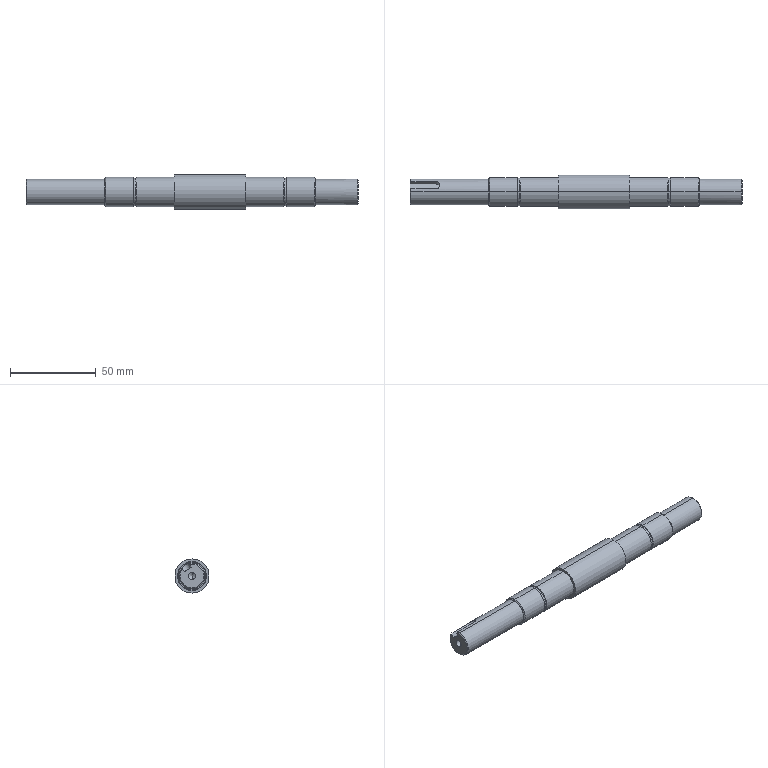Part | SolidWorks | features BaseBody 1 | 1 solid | 53 faces | box 194 x 20 x 20 mm | volume 43584 mm3 | cylinder 21 | plane 13 | cone 11 | spline 8 | commonest cylinder face diameters 17 x8 15 x4 16 x4 4.2 x2 20 x2 5 x1